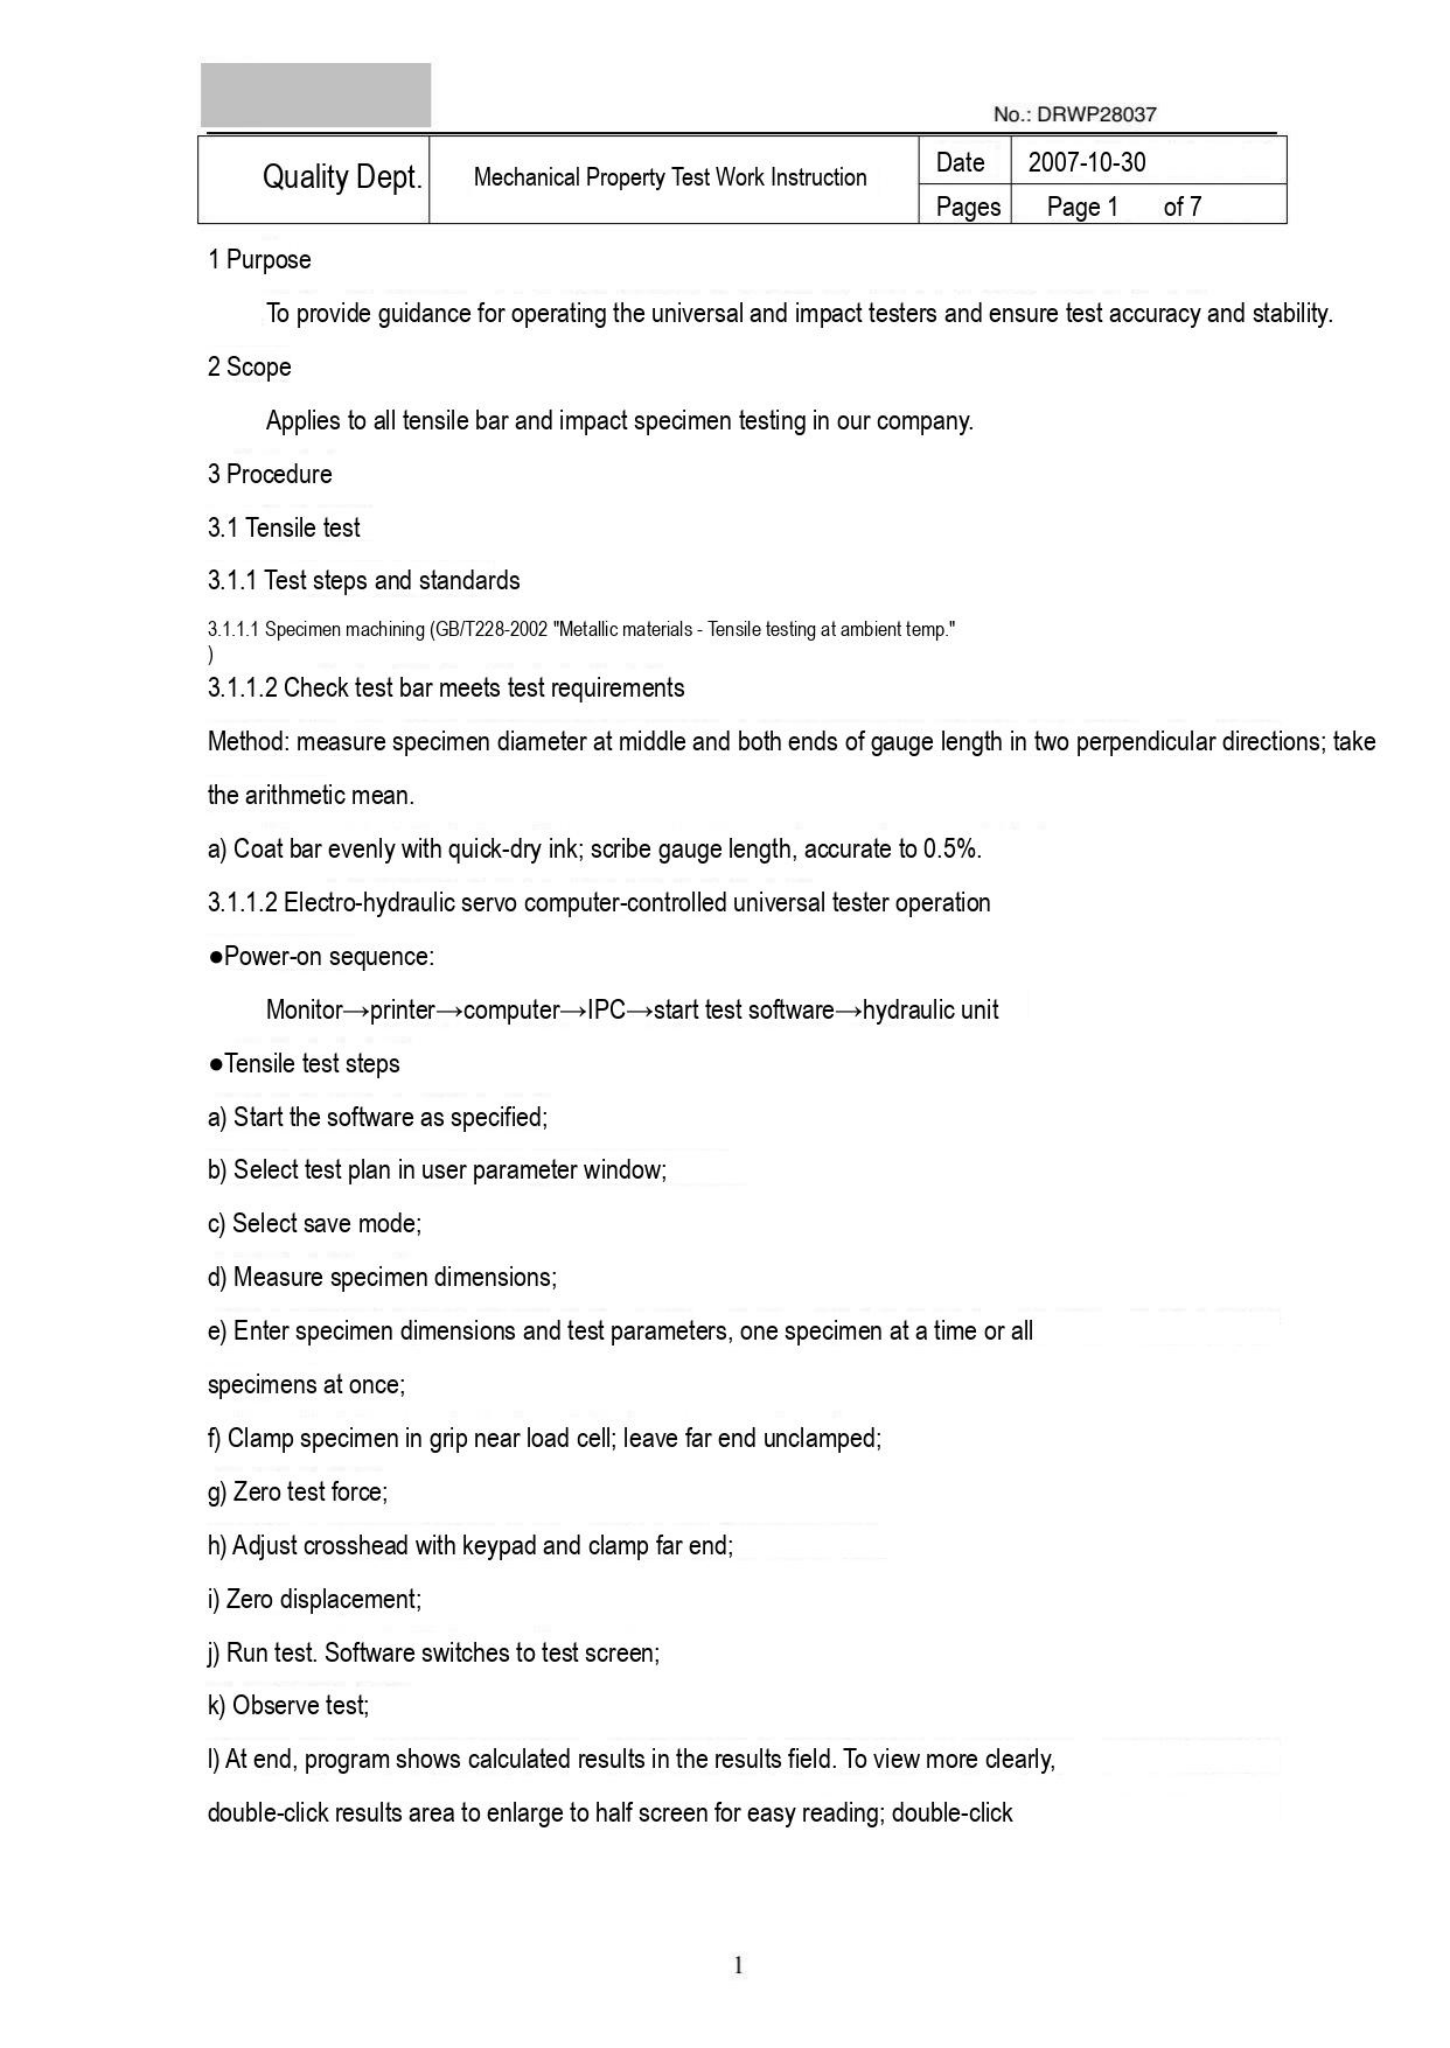No.: DRWP28037

| Quality Dept. | Mechanical Property Test Work Instruction | Date | 2007-10-30 |
|---|---|---|---|
| | | Pages | Page 1 of 7 |

1 Purpose

To provide guidance for operating the universal and impact testers and ensure test accuracy and stability.

2 Scope

Applies to all tensile bar and impact specimen testing in our company.

3 Procedure

3.1 Tensile test

3.1.1 Test steps and standards

3.1.1.1 Specimen machining (GB/T228-2002 "Metallic materials - Tensile testing at ambient temp."
)

3.1.1.2 Check test bar meets test requirements

Method: measure specimen diameter at middle and both ends of gauge length in two perpendicular directions; take the arithmetic mean.

a) Coat bar evenly with quick-dry ink; scribe gauge length, accurate to 0.5%.

3.1.1.2 Electro-hydraulic servo computer-controlled universal tester operation

●Power-on sequence:

Monitor→printer→computer→IPC→start test software→hydraulic unit

●Tensile test steps

a) Start the software as specified;

b) Select test plan in user parameter window;

c) Select save mode;

d) Measure specimen dimensions;

e) Enter specimen dimensions and test parameters, one specimen at a time or all specimens at once;

f) Clamp specimen in grip near load cell; leave far end unclamped;

g) Zero test force;

h) Adjust crosshead with keypad and clamp far end;

i) Zero displacement;

j) Run test. Software switches to test screen;

k) Observe test;

l) At end, program shows calculated results in the results field. To view more clearly, double-click results area to enlarge to half screen for easy reading; double-click

1
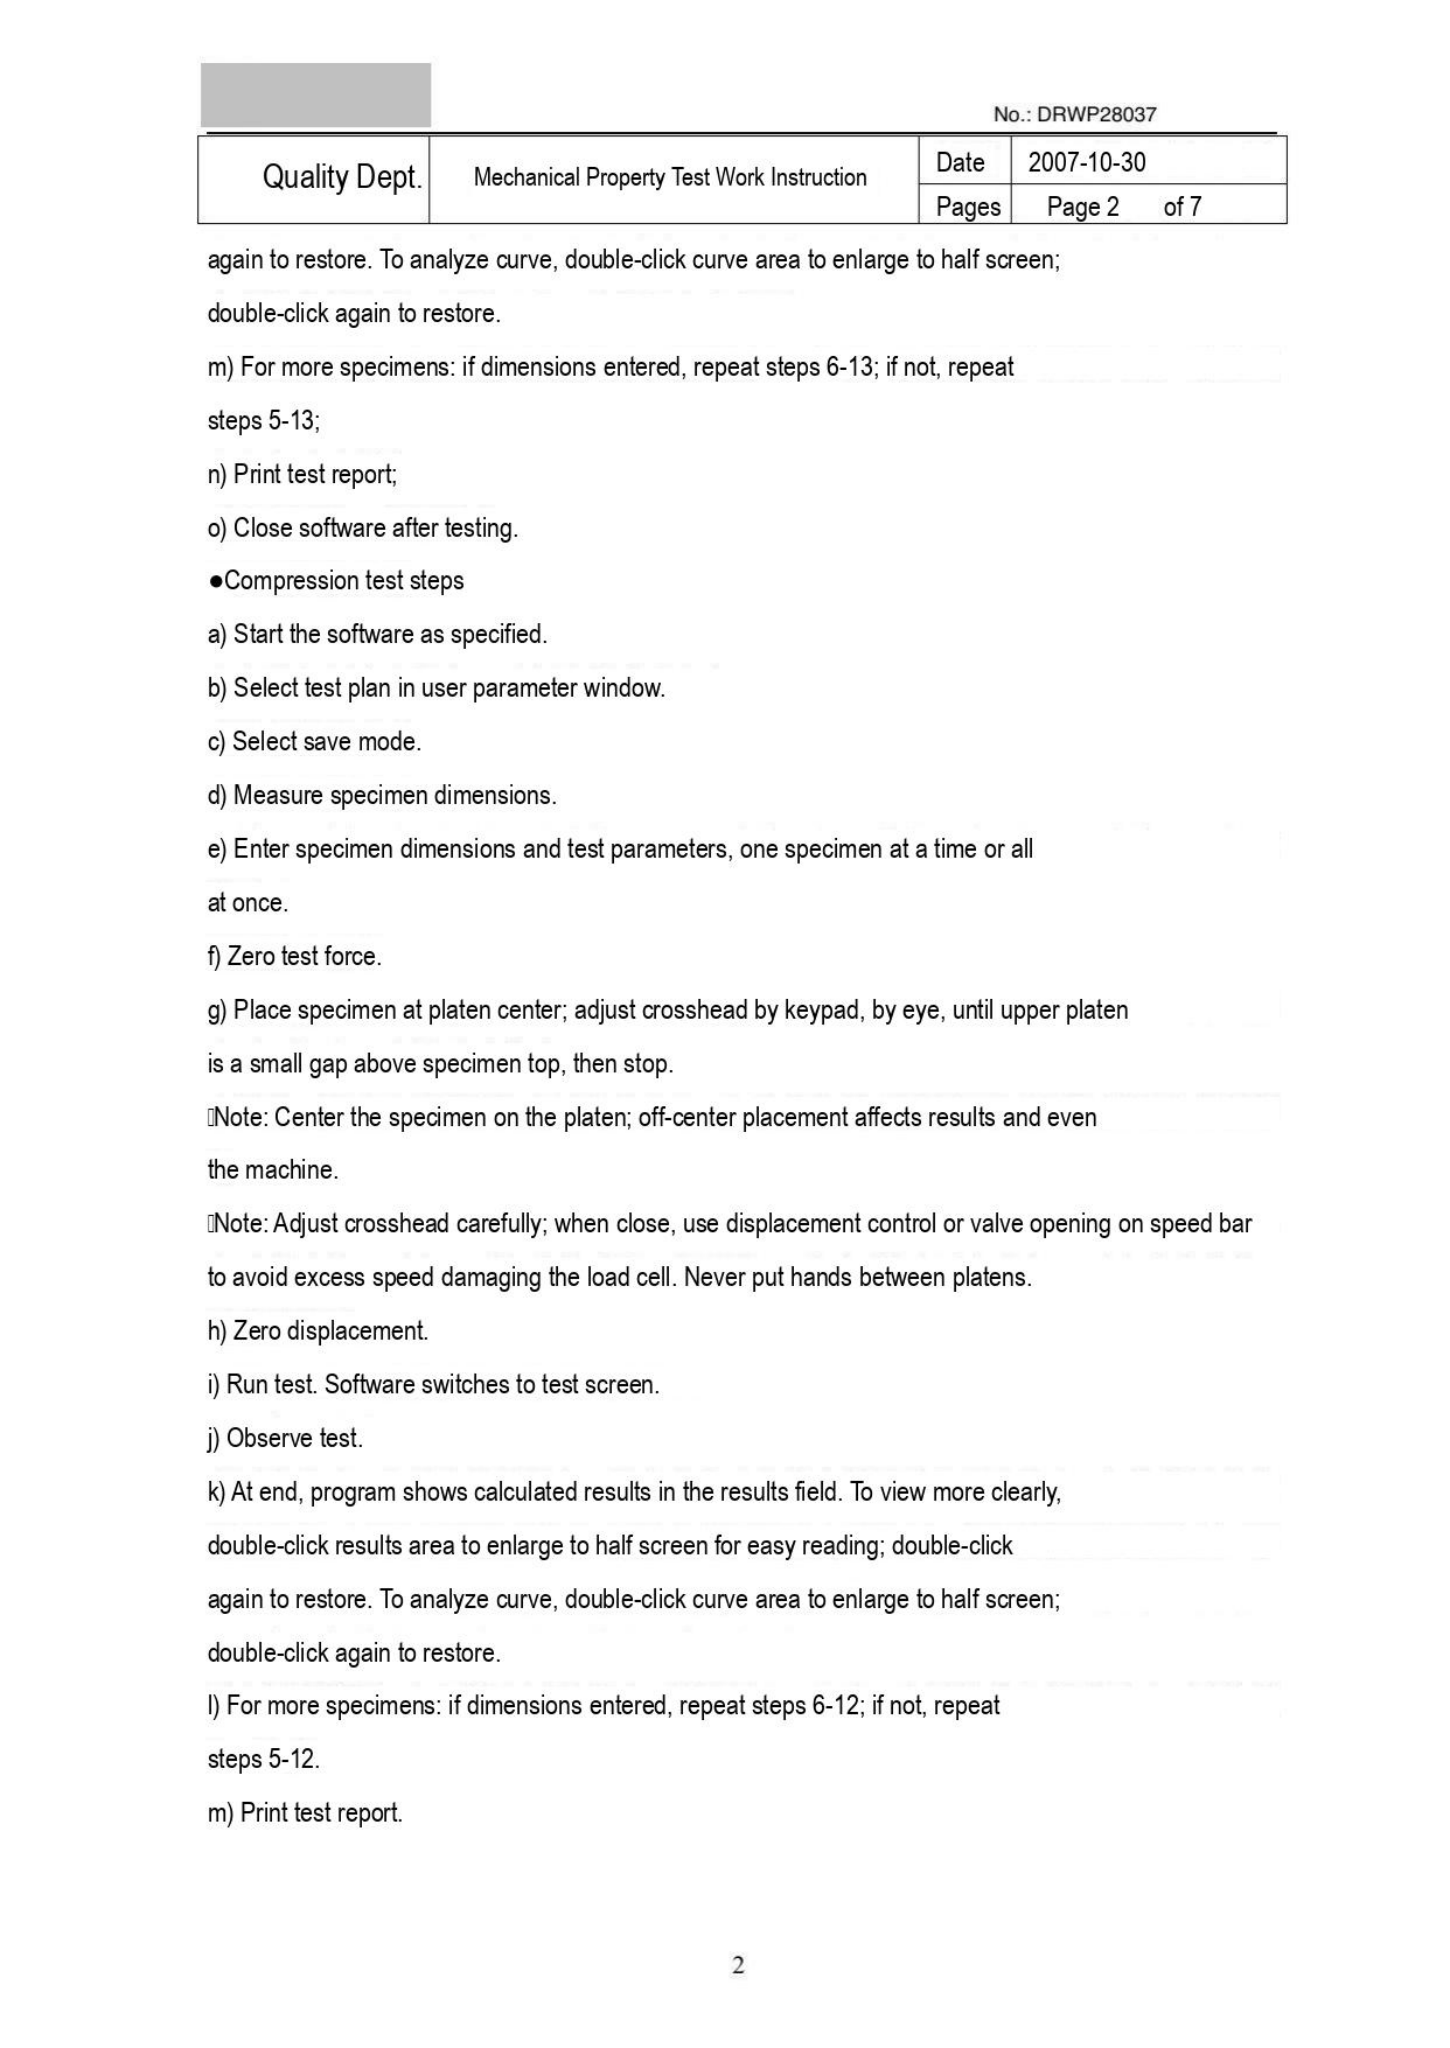No.: DRWP28037

| Quality Dept. | Mechanical Property Test Work Instruction | Date | 2007-10-30 |
|---|---|---|---|
| | | Pages | Page 2 of 7 |

again to restore. To analyze curve, double-click curve area to enlarge to half screen; double-click again to restore.

m) For more specimens: if dimensions entered, repeat steps 6-13; if not, repeat steps 5-13;

n) Print test report;

o) Close software after testing.

●Compression test steps

a) Start the software as specified.

b) Select test plan in user parameter window.

c) Select save mode.

d) Measure specimen dimensions.

e) Enter specimen dimensions and test parameters, one specimen at a time or all at once.

f) Zero test force.

g) Place specimen at platen center; adjust crosshead by keypad, by eye, until upper platen is a small gap above specimen top, then stop.

Note: Center the specimen on the platen; off-center placement affects results and even the machine.

Note: Adjust crosshead carefully; when close, use displacement control or valve opening on speed bar to avoid excess speed damaging the load cell. Never put hands between platens.

h) Zero displacement.

i) Run test. Software switches to test screen.

j) Observe test.

k) At end, program shows calculated results in the results field. To view more clearly, double-click results area to enlarge to half screen for easy reading; double-click again to restore. To analyze curve, double-click curve area to enlarge to half screen; double-click again to restore.

l) For more specimens: if dimensions entered, repeat steps 6-12; if not, repeat steps 5-12.

m) Print test report.

2
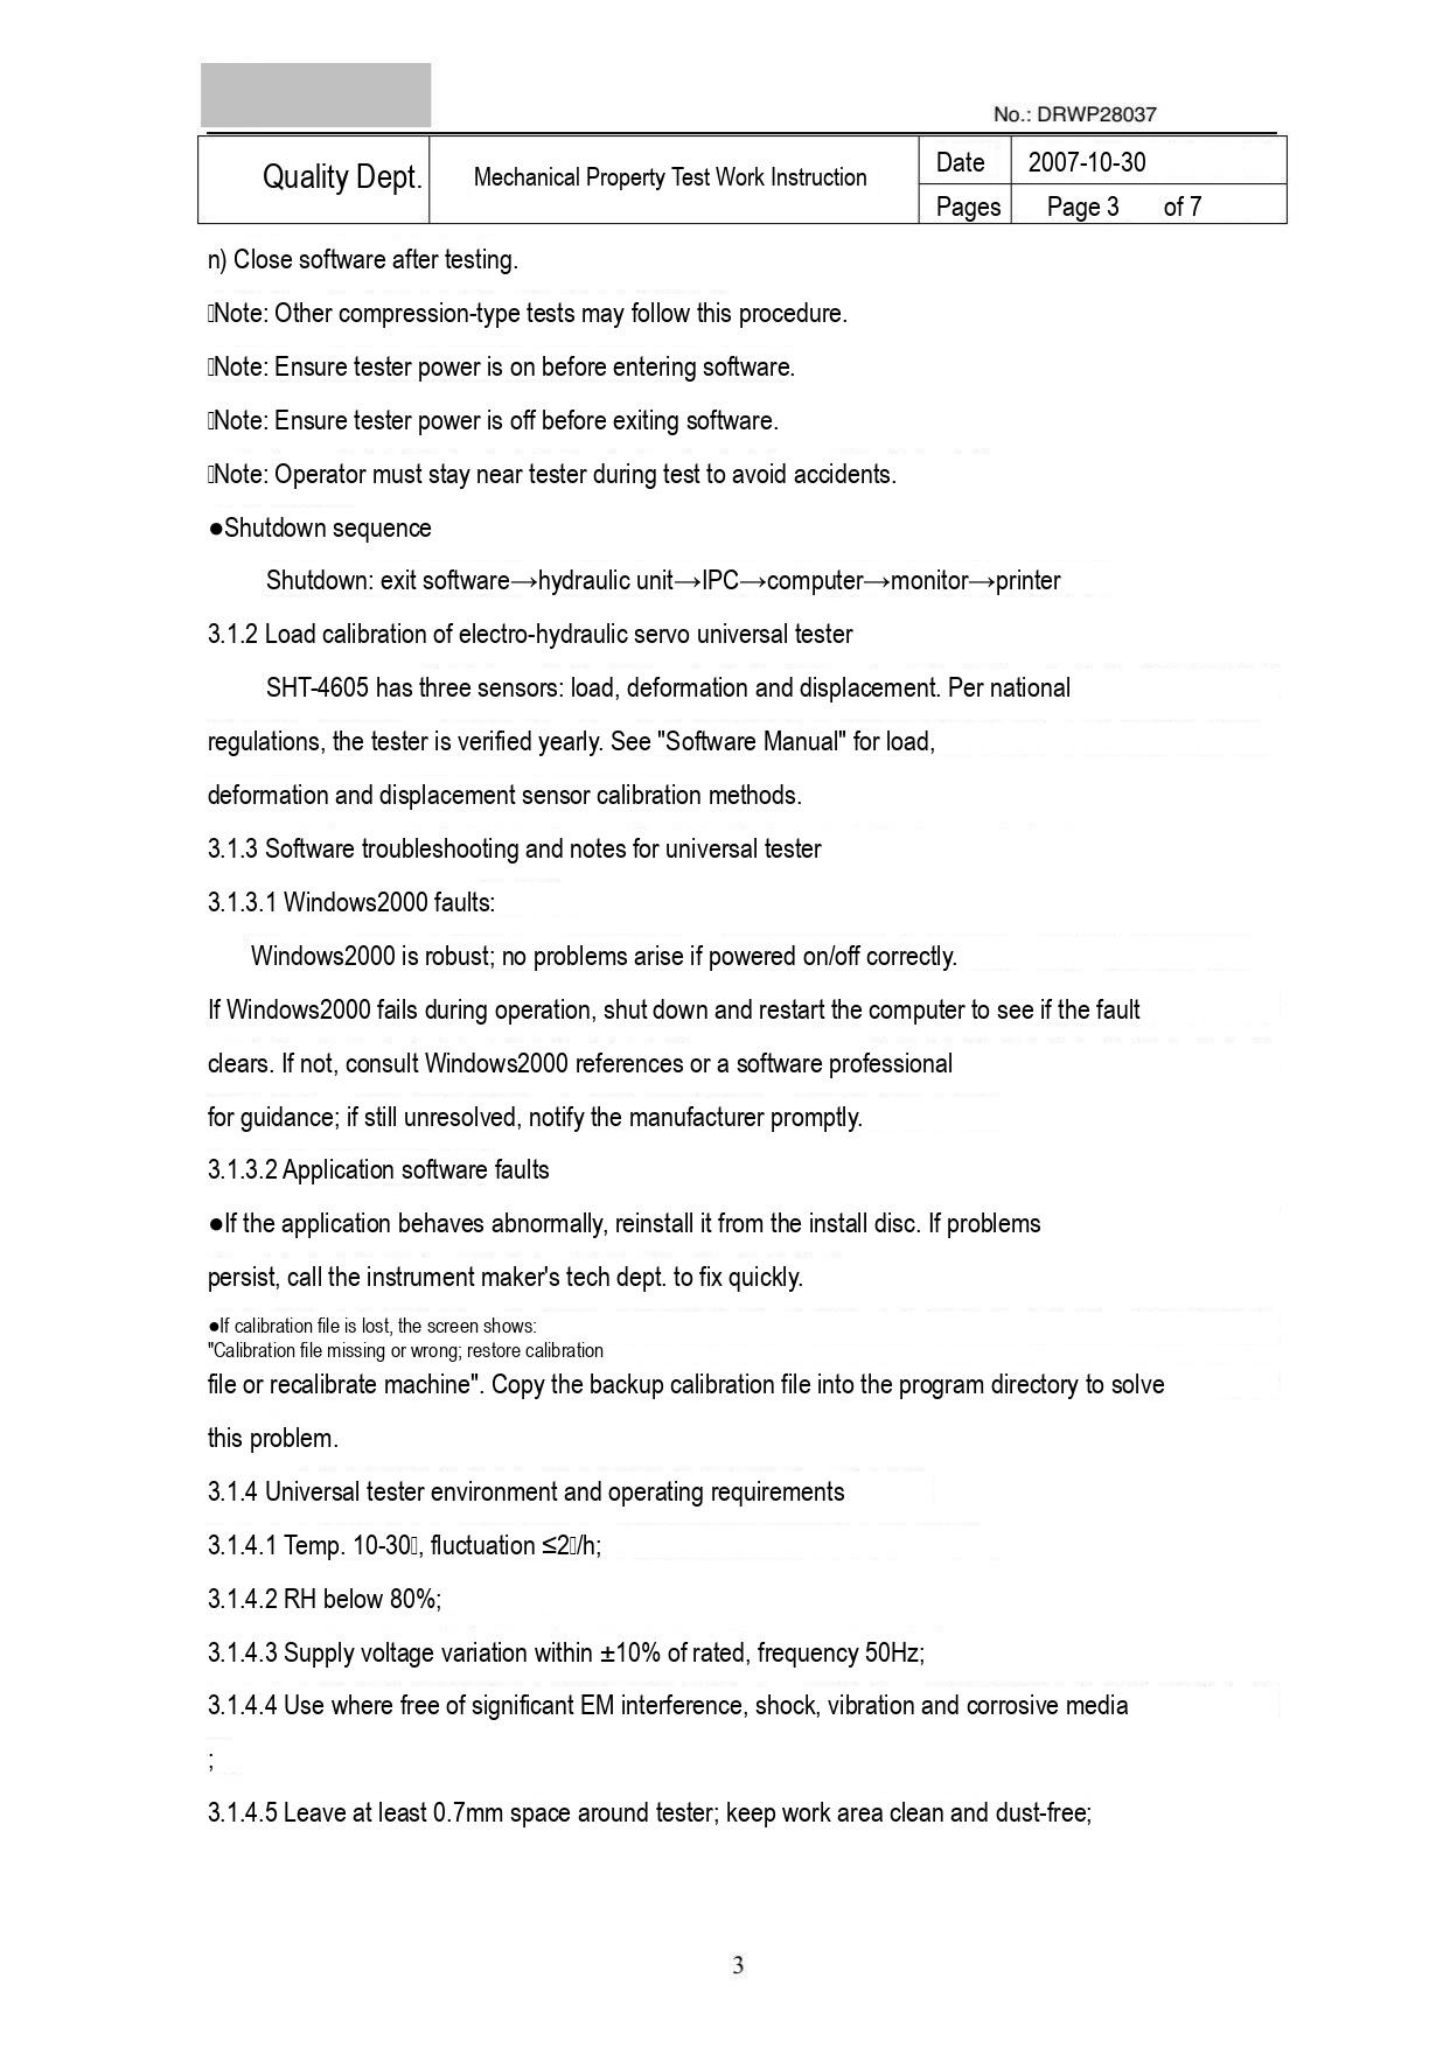No.: DRWP28037

| Quality Dept. | Mechanical Property Test Work Instruction | Date | 2007-10-30 |
|---|---|---|---|
| | | Pages | Page 3 of 7 |

n) Close software after testing.

Note: Other compression-type tests may follow this procedure.

Note: Ensure tester power is on before entering software.

Note: Ensure tester power is off before exiting software.

Note: Operator must stay near tester during test to avoid accidents.

●Shutdown sequence

Shutdown: exit software→hydraulic unit→IPC→computer→monitor→printer

3.1.2 Load calibration of electro-hydraulic servo universal tester

SHT-4605 has three sensors: load, deformation and displacement. Per national regulations, the tester is verified yearly. See "Software Manual" for load, deformation and displacement sensor calibration methods.

3.1.3 Software troubleshooting and notes for universal tester

3.1.3.1 Windows2000 faults:

Windows2000 is robust; no problems arise if powered on/off correctly.

If Windows2000 fails during operation, shut down and restart the computer to see if the fault clears. If not, consult Windows2000 references or a software professional for guidance; if still unresolved, notify the manufacturer promptly.

3.1.3.2 Application software faults

●If the application behaves abnormally, reinstall it from the install disc. If problems persist, call the instrument maker's tech dept. to fix quickly.

●If calibration file is lost, the screen shows:
"Calibration file missing or wrong; restore calibration file or recalibrate machine". Copy the backup calibration file into the program directory to solve this problem.

3.1.4 Universal tester environment and operating requirements

3.1.4.1 Temp. 10-30, fluctuation ≤2/h;

3.1.4.2 RH below 80%;

3.1.4.3 Supply voltage variation within ±10% of rated, frequency 50Hz;

3.1.4.4 Use where free of significant EM interference, shock, vibration and corrosive media
;

3.1.4.5 Leave at least 0.7mm space around tester; keep work area clean and dust-free;

3
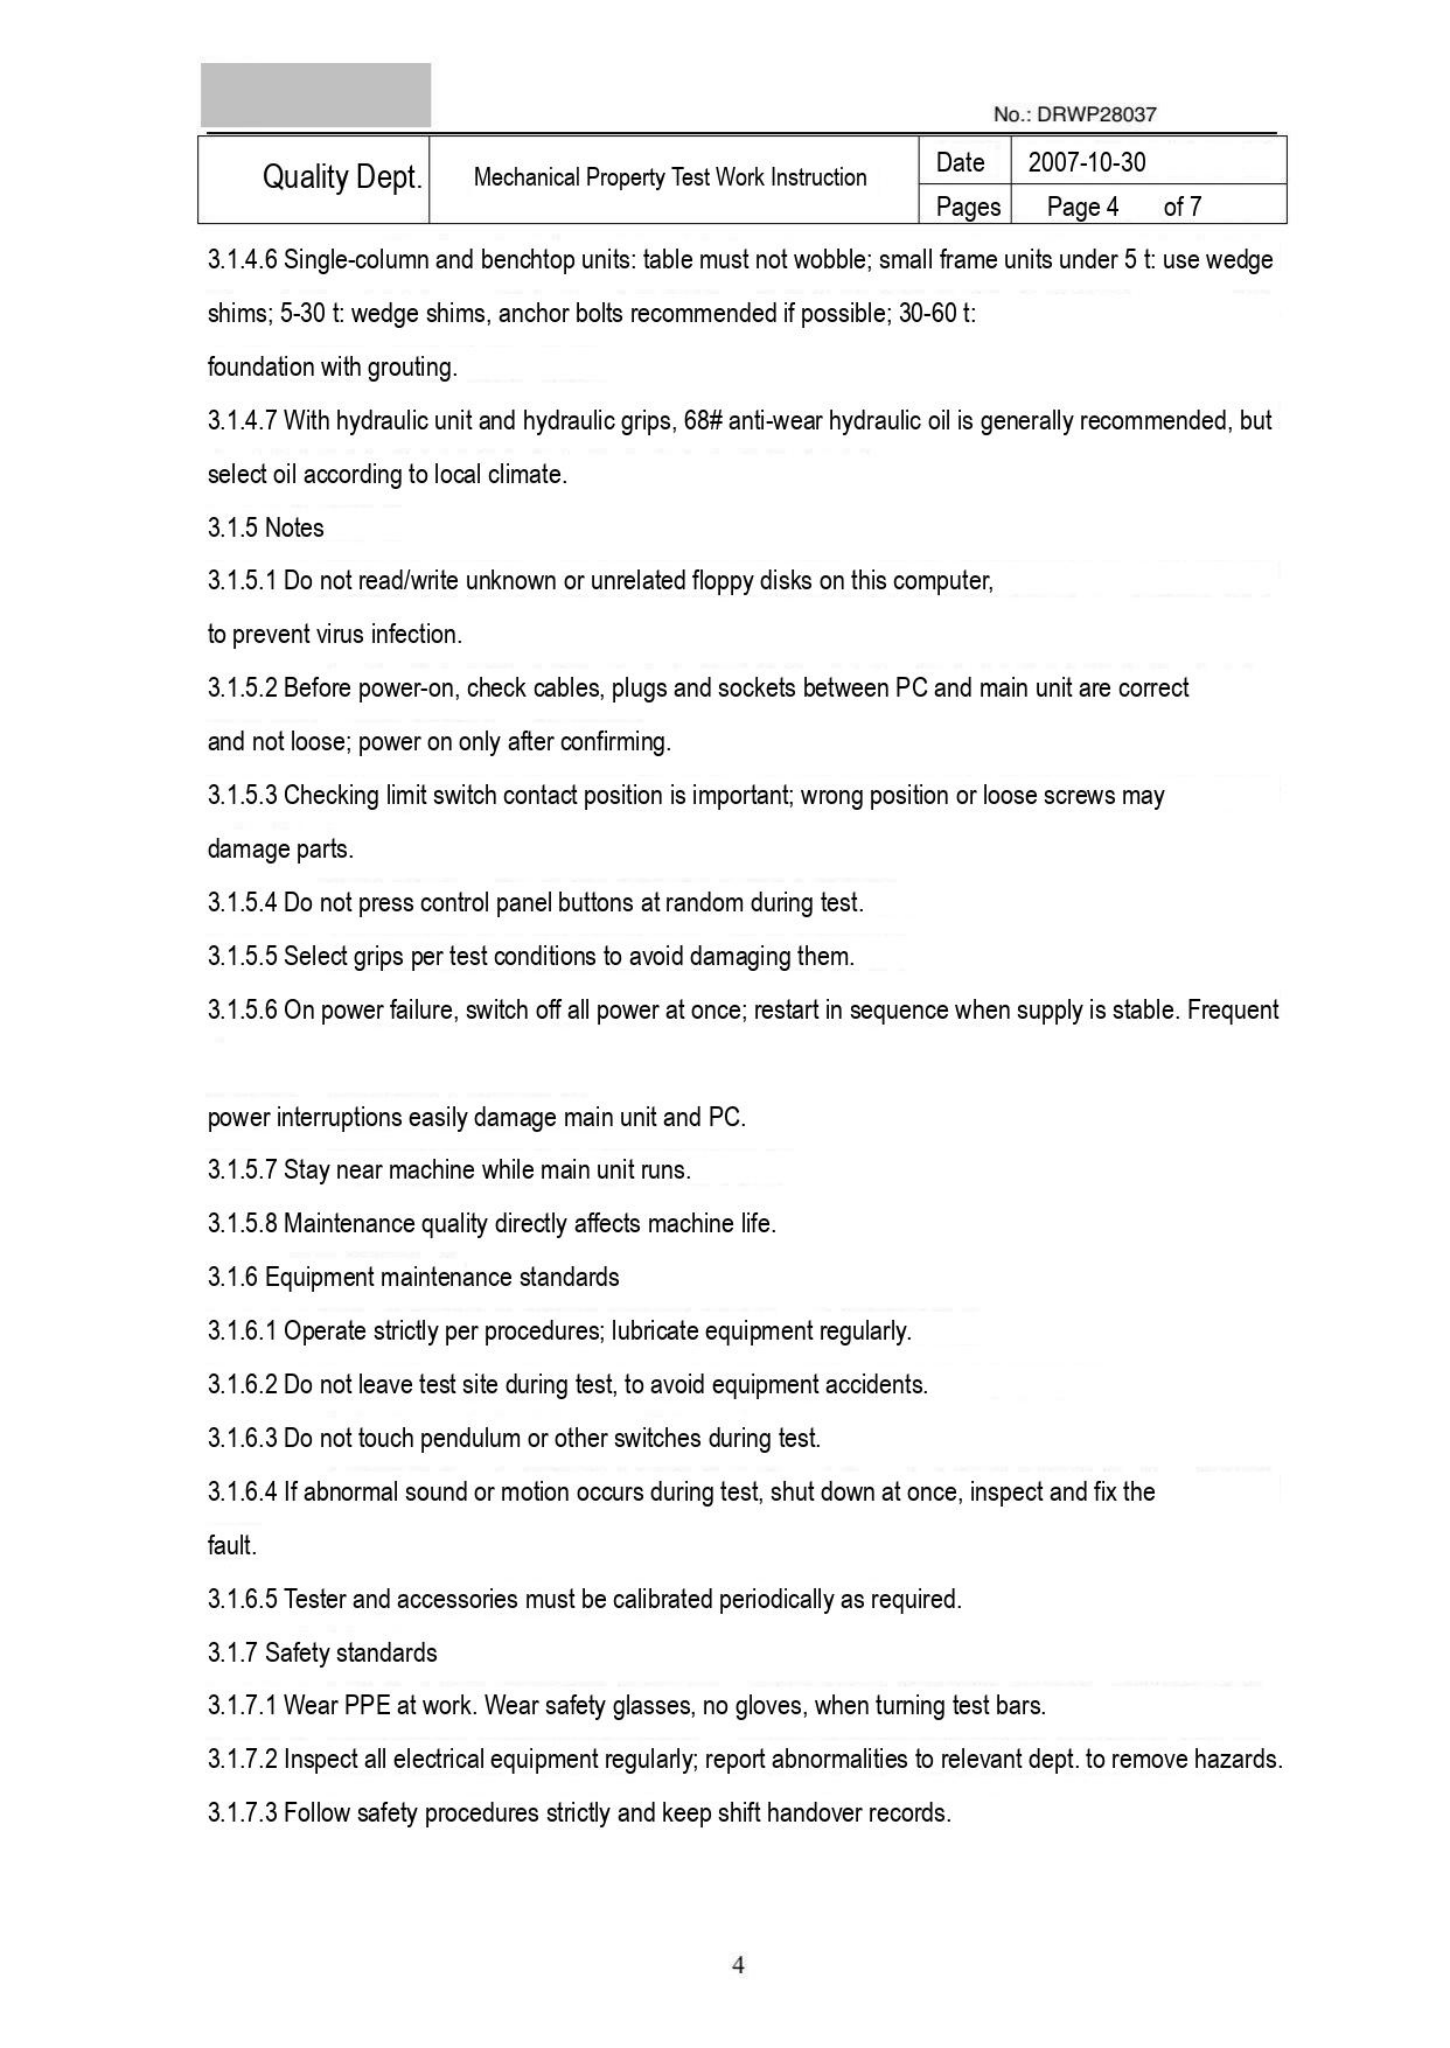No.: DRWP28037

| Quality Dept. | Mechanical Property Test Work Instruction | Date | 2007-10-30 |
|---|---|---|---|
| | | Pages | Page 4 of 7 |

3.1.4.6 Single-column and benchtop units: table must not wobble; small frame units under 5 t: use wedge shims; 5-30 t: wedge shims, anchor bolts recommended if possible; 30-60 t:
foundation with grouting.
3.1.4.7 With hydraulic unit and hydraulic grips, 68# anti-wear hydraulic oil is generally recommended, but select oil according to local climate.
3.1.5 Notes
3.1.5.1 Do not read/write unknown or unrelated floppy disks on this computer,
to prevent virus infection.
3.1.5.2 Before power-on, check cables, plugs and sockets between PC and main unit are correct
and not loose; power on only after confirming.
3.1.5.3 Checking limit switch contact position is important; wrong position or loose screws may
damage parts.
3.1.5.4 Do not press control panel buttons at random during test.
3.1.5.5 Select grips per test conditions to avoid damaging them.
3.1.5.6 On power failure, switch off all power at once; restart in sequence when supply is stable. Frequent

power interruptions easily damage main unit and PC.
3.1.5.7 Stay near machine while main unit runs.
3.1.5.8 Maintenance quality directly affects machine life.
3.1.6 Equipment maintenance standards
3.1.6.1 Operate strictly per procedures; lubricate equipment regularly.
3.1.6.2 Do not leave test site during test, to avoid equipment accidents.
3.1.6.3 Do not touch pendulum or other switches during test.
3.1.6.4 If abnormal sound or motion occurs during test, shut down at once, inspect and fix the
fault.
3.1.6.5 Tester and accessories must be calibrated periodically as required.
3.1.7 Safety standards
3.1.7.1 Wear PPE at work. Wear safety glasses, no gloves, when turning test bars.
3.1.7.2 Inspect all electrical equipment regularly; report abnormalities to relevant dept. to remove hazards.
3.1.7.3 Follow safety procedures strictly and keep shift handover records.

4
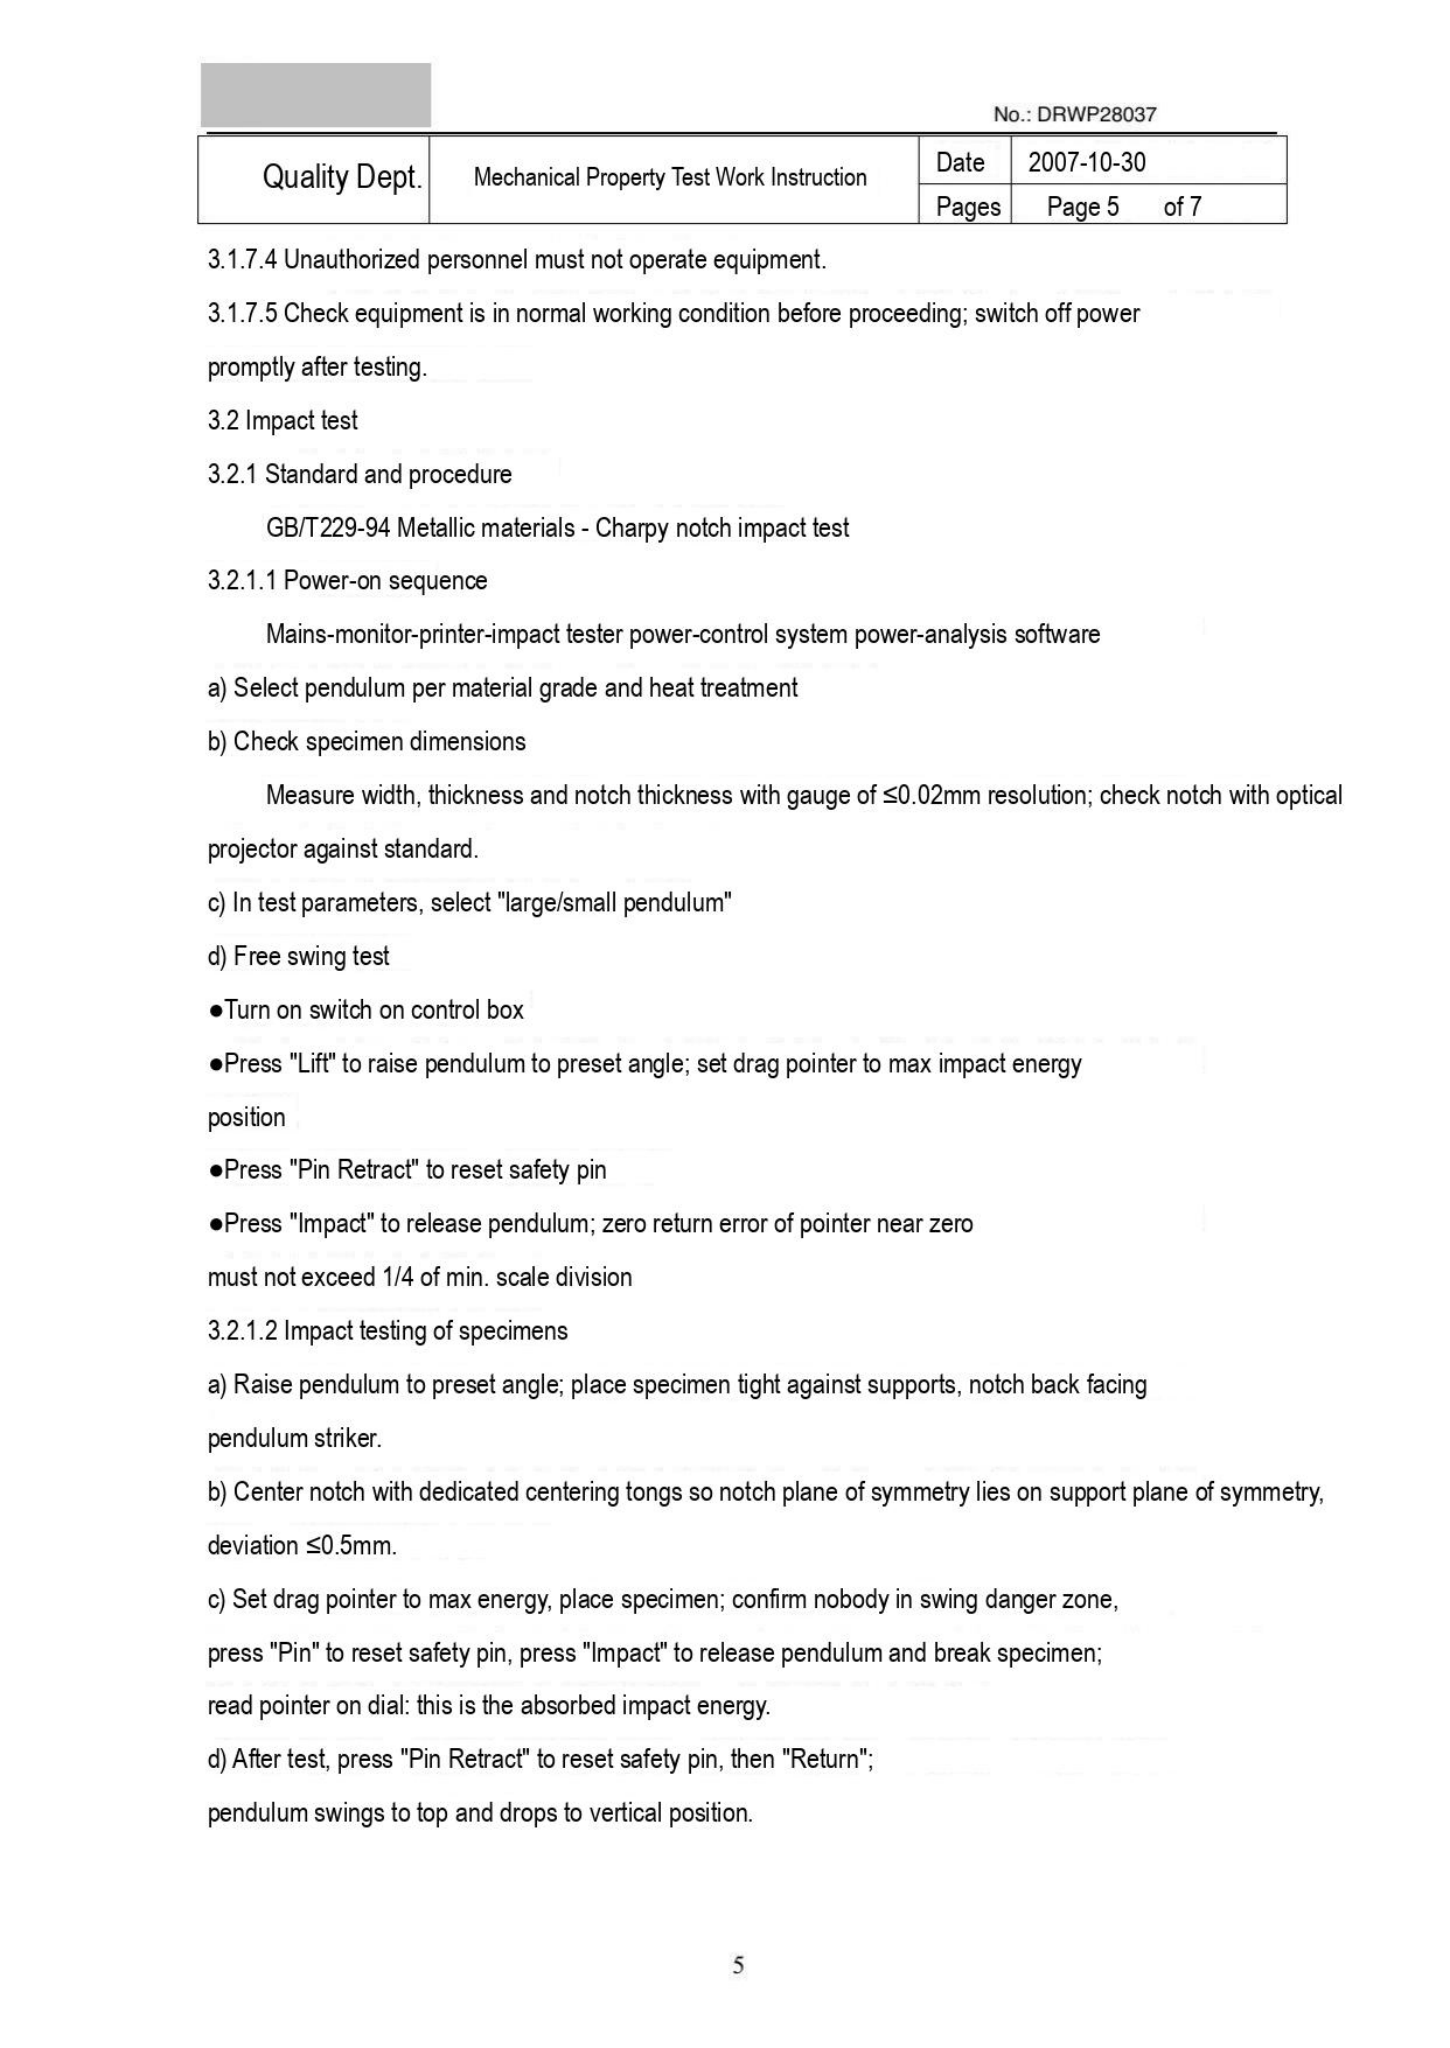No.: DRWP28037

| Quality Dept. | Mechanical Property Test Work Instruction | Date | 2007-10-30 |
|---|---|---|---|
| | | Pages | Page 5 of 7 |

3.1.7.4 Unauthorized personnel must not operate equipment.

3.1.7.5 Check equipment is in normal working condition before proceeding; switch off power promptly after testing.

3.2 Impact test

3.2.1 Standard and procedure

GB/T229-94 Metallic materials - Charpy notch impact test

3.2.1.1 Power-on sequence

Mains-monitor-printer-impact tester power-control system power-analysis software

a) Select pendulum per material grade and heat treatment

b) Check specimen dimensions

Measure width, thickness and notch thickness with gauge of ≤0.02mm resolution; check notch with optical projector against standard.

c) In test parameters, select "large/small pendulum"

d) Free swing test

●Turn on switch on control box

●Press "Lift" to raise pendulum to preset angle; set drag pointer to max impact energy position

●Press "Pin Retract" to reset safety pin

●Press "Impact" to release pendulum; zero return error of pointer near zero must not exceed 1/4 of min. scale division

3.2.1.2 Impact testing of specimens

a) Raise pendulum to preset angle; place specimen tight against supports, notch back facing pendulum striker.

b) Center notch with dedicated centering tongs so notch plane of symmetry lies on support plane of symmetry, deviation ≤0.5mm.

c) Set drag pointer to max energy, place specimen; confirm nobody in swing danger zone, press "Pin" to reset safety pin, press "Impact" to release pendulum and break specimen; read pointer on dial: this is the absorbed impact energy.

d) After test, press "Pin Retract" to reset safety pin, then "Return"; pendulum swings to top and drops to vertical position.

5
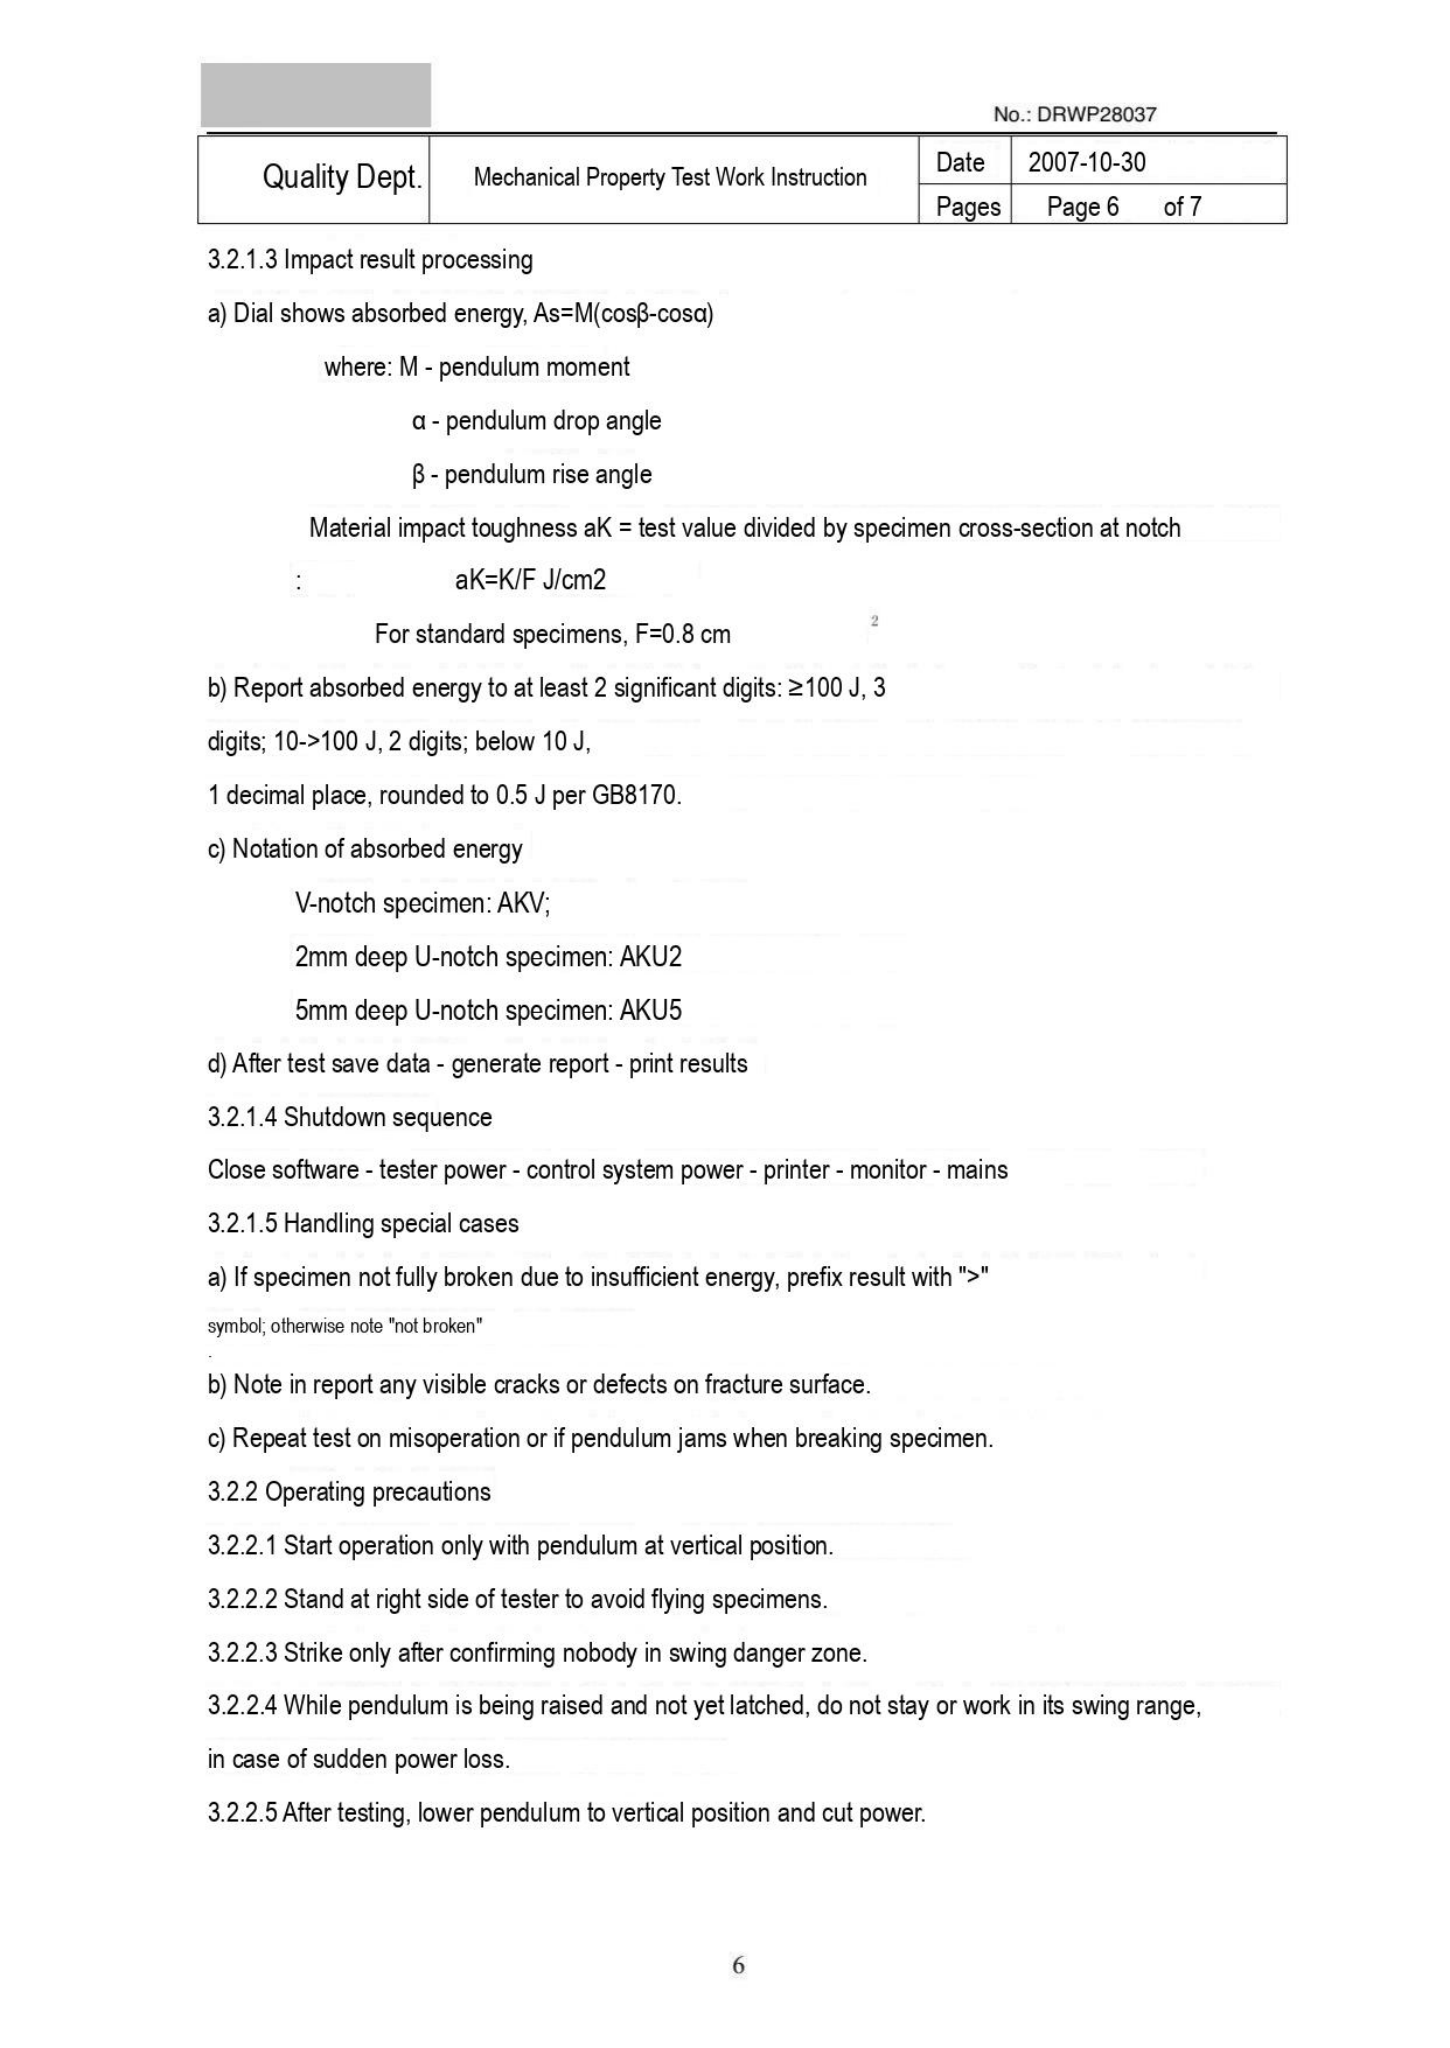No.: DRWP28037

| Quality Dept. | Mechanical Property Test Work Instruction | Date | 2007-10-30 |
|---|---|---|---|
| | | Pages | Page 6 of 7 |

3.2.1.3 Impact result processing

a) Dial shows absorbed energy, As=M(cosβ-cosα)

where: M - pendulum moment

α - pendulum drop angle

β - pendulum rise angle

Material impact toughness aK = test value divided by specimen cross-section at notch

: aK=K/F J/cm2

For standard specimens, F=0.8 cm 2

b) Report absorbed energy to at least 2 significant digits: ≥100 J, 3

digits; 10->100 J, 2 digits; below 10 J,

1 decimal place, rounded to 0.5 J per GB8170.

c) Notation of absorbed energy

V-notch specimen: AKV;

2mm deep U-notch specimen: AKU2

5mm deep U-notch specimen: AKU5

d) After test save data - generate report - print results

3.2.1.4 Shutdown sequence

Close software - tester power - control system power - printer - monitor - mains

3.2.1.5 Handling special cases

a) If specimen not fully broken due to insufficient energy, prefix result with ">"

symbol; otherwise note "not broken"

b) Note in report any visible cracks or defects on fracture surface.

c) Repeat test on misoperation or if pendulum jams when breaking specimen.

3.2.2 Operating precautions

3.2.2.1 Start operation only with pendulum at vertical position.

3.2.2.2 Stand at right side of tester to avoid flying specimens.

3.2.2.3 Strike only after confirming nobody in swing danger zone.

3.2.2.4 While pendulum is being raised and not yet latched, do not stay or work in its swing range, in case of sudden power loss.

3.2.2.5 After testing, lower pendulum to vertical position and cut power.

6
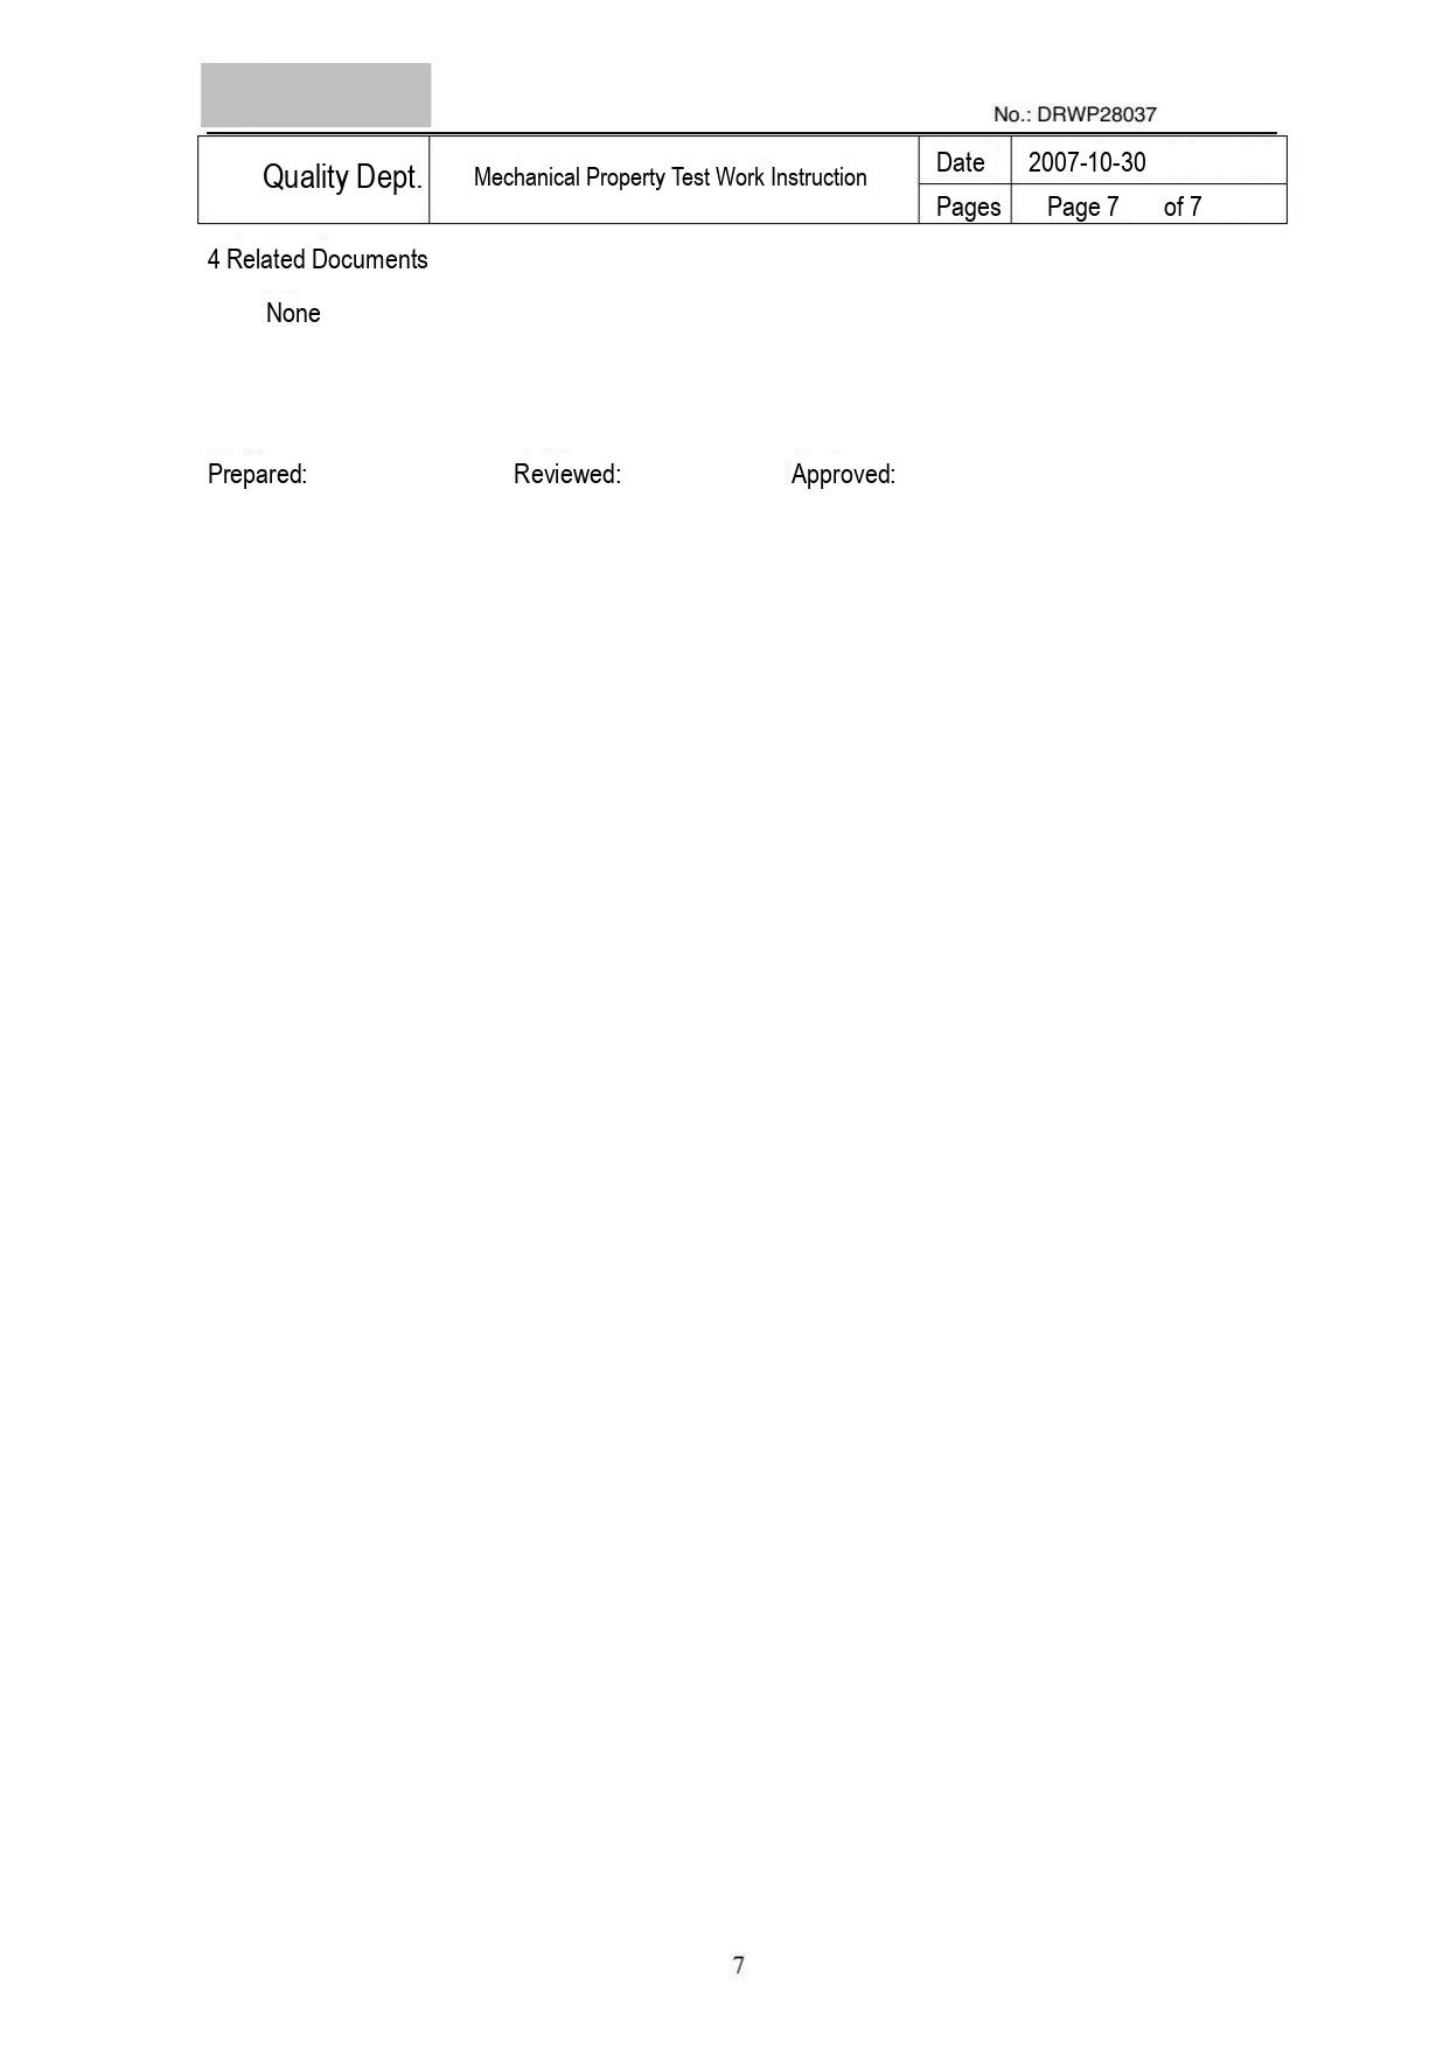No.: DRWP28037

| Quality Dept. | Mechanical Property Test Work Instruction | Date | 2007-10-30 |
|---|---|---|---|
| | | Pages | Page 7 of 7 |

4 Related Documents

None

Prepared: Reviewed: Approved:

7